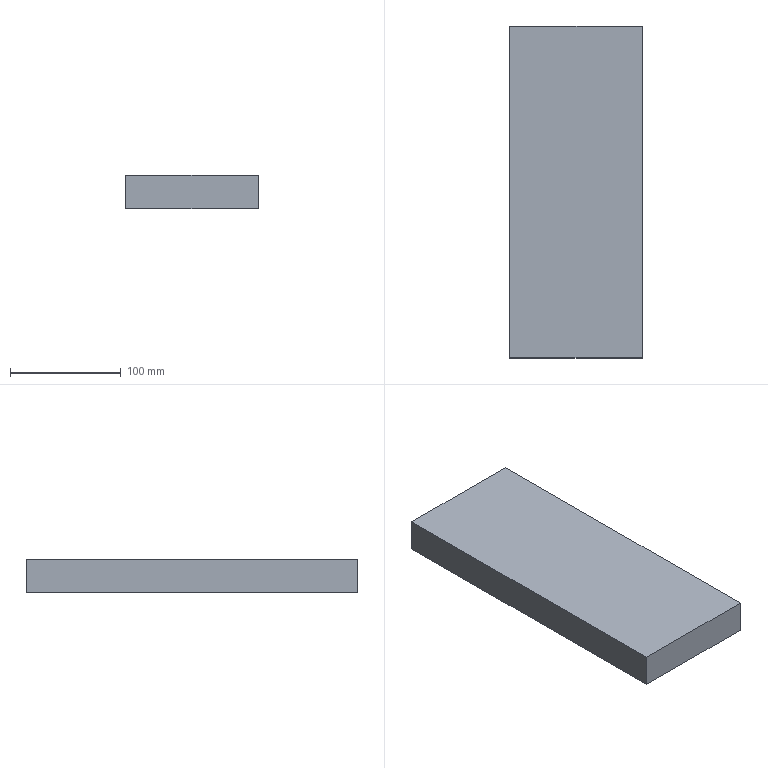Part | SolidWorks | features Extrusion 1 | 1 solid | 6 faces | box 120 x 300 x 30 mm | volume 1080000 mm3 | plane 6
STEP:
#1=CARTESIAN_POINT('',(0.,300.,0.));
#2=VERTEX_POINT('',#1);
#3=CARTESIAN_POINT('',(0.,0.,0.));
#4=VERTEX_POINT('',#3);
#5=CARTESIAN_POINT('',(0.,0.,0.));
#6=DIRECTION('',(0.,-1.,0.));
#7=VECTOR('',#6,1000.);
#8=LINE('',#5,#7);
#9=EDGE_CURVE('',#2,#4,#8,.T.);
#10=ORIENTED_EDGE('',*,*,#9,.T.);
#11=CARTESIAN_POINT('',(0.,0.,30.));
#12=VERTEX_POINT('',#11);
#13=CARTESIAN_POINT('',(0.,0.,30.));
#14=DIRECTION('',(0.,0.,-1.));
#15=VECTOR('',#14,1000.);
#16=LINE('',#13,#15);
#17=EDGE_CURVE('',#12,#4,#16,.T.);
#18=ORIENTED_EDGE('',*,*,#17,.F.);
#19=CARTESIAN_POINT('',(0.,300.,30.));
#20=VERTEX_POINT('',#19);
#21=CARTESIAN_POINT('',(0.,0.,30.));
#22=DIRECTION('',(0.,-1.,0.));
#23=VECTOR('',#22,1000.);
#24=LINE('',#21,#23);
#25=EDGE_CURVE('',#20,#12,#24,.T.);
#26=ORIENTED_EDGE('',*,*,#25,.F.);
#27=CARTESIAN_POINT('',(0.,300.,30.));
#28=DIRECTION('',(0.,0.,-1.));
#29=VECTOR('',#28,1000.);
#30=LINE('',#27,#29);
#31=EDGE_CURVE('',#20,#2,#30,.T.);
#32=ORIENTED_EDGE('',*,*,#31,.T.);
#33=EDGE_LOOP('',(#10,#18,#26,#32));
#34=FACE_OUTER_BOUND('',#33,.T.);
#35=CARTESIAN_POINT('',(0.,0.,30.));
#36=DIRECTION('',(1.,0.,0.));
#37=DIRECTION('',(0.,1.,0.));
#38=AXIS2_PLACEMENT_3D('',#35,#36,#37);
#39=PLANE('',#38);
#40=ADVANCED_FACE('',(#34),#39,.F.);
#41=CARTESIAN_POINT('',(120.,0.,0.));
#42=VERTEX_POINT('',#41);
#43=CARTESIAN_POINT('',(0.,0.,0.));
#44=DIRECTION('',(1.,0.,0.));
#45=VECTOR('',#44,1000.);
#46=LINE('',#43,#45);
#47=EDGE_CURVE('',#4,#42,#46,.T.);
#48=ORIENTED_EDGE('',*,*,#47,.T.);
#49=CARTESIAN_POINT('',(120.,0.,30.));
#50=VERTEX_POINT('',#49);
#51=CARTESIAN_POINT('',(120.,0.,30.));
#52=DIRECTION('',(0.,0.,-1.));
#53=VECTOR('',#52,1000.);
#54=LINE('',#51,#53);
#55=EDGE_CURVE('',#50,#42,#54,.T.);
#56=ORIENTED_EDGE('',*,*,#55,.F.);
#57=CARTESIAN_POINT('',(0.,0.,30.));
#58=DIRECTION('',(1.,0.,0.));
#59=VECTOR('',#58,1000.);
#60=LINE('',#57,#59);
#61=EDGE_CURVE('',#12,#50,#60,.T.);
#62=ORIENTED_EDGE('',*,*,#61,.F.);
#63=ORIENTED_EDGE('',*,*,#17,.T.);
#64=EDGE_LOOP('',(#48,#56,#62,#63));
#65=FACE_OUTER_BOUND('',#64,.T.);
#66=CARTESIAN_POINT('',(0.,0.,30.));
#67=DIRECTION('',(0.,1.,0.));
#68=DIRECTION('',(0.,0.,1.));
#69=AXIS2_PLACEMENT_3D('',#66,#67,#68);
#70=PLANE('',#69);
#71=ADVANCED_FACE('',(#65),#70,.F.);
#72=CARTESIAN_POINT('',(120.,300.,0.));
#73=VERTEX_POINT('',#72);
#74=CARTESIAN_POINT('',(120.,0.,0.));
#75=DIRECTION('',(0.,1.,0.));
#76=VECTOR('',#75,1000.);
#77=LINE('',#74,#76);
#78=EDGE_CURVE('',#42,#73,#77,.T.);
#79=ORIENTED_EDGE('',*,*,#78,.T.);
#80=CARTESIAN_POINT('',(120.,300.,30.));
#81=VERTEX_POINT('',#80);
#82=CARTESIAN_POINT('',(120.,300.,30.));
#83=DIRECTION('',(0.,0.,-1.));
#84=VECTOR('',#83,1000.);
#85=LINE('',#82,#84);
#86=EDGE_CURVE('',#81,#73,#85,.T.);
#87=ORIENTED_EDGE('',*,*,#86,.F.);
#88=CARTESIAN_POINT('',(120.,0.,30.));
#89=DIRECTION('',(0.,1.,0.));
#90=VECTOR('',#89,1000.);
#91=LINE('',#88,#90);
#92=EDGE_CURVE('',#50,#81,#91,.T.);
#93=ORIENTED_EDGE('',*,*,#92,.F.);
#94=ORIENTED_EDGE('',*,*,#55,.T.);
#95=EDGE_LOOP('',(#79,#87,#93,#94));
#96=FACE_OUTER_BOUND('',#95,.T.);
#97=CARTESIAN_POINT('',(120.,0.,30.));
#98=DIRECTION('',(-1.,0.,0.));
#99=DIRECTION('',(0.,-1.,0.));
#100=AXIS2_PLACEMENT_3D('',#97,#98,#99);
#101=PLANE('',#100);
#102=ADVANCED_FACE('',(#96),#101,.F.);
#103=CARTESIAN_POINT('',(0.,300.,0.));
#104=DIRECTION('',(-1.,0.,0.));
#105=VECTOR('',#104,1000.);
#106=LINE('',#103,#105);
#107=EDGE_CURVE('',#73,#2,#106,.T.);
#108=ORIENTED_EDGE('',*,*,#107,.T.);
#109=ORIENTED_EDGE('',*,*,#31,.F.);
#110=CARTESIAN_POINT('',(0.,300.,30.));
#111=DIRECTION('',(-1.,0.,0.));
#112=VECTOR('',#111,1000.);
#113=LINE('',#110,#112);
#114=EDGE_CURVE('',#81,#20,#113,.T.);
#115=ORIENTED_EDGE('',*,*,#114,.F.);
#116=ORIENTED_EDGE('',*,*,#86,.T.);
#117=EDGE_LOOP('',(#108,#109,#115,#116));
#118=FACE_OUTER_BOUND('',#117,.T.);
#119=CARTESIAN_POINT('',(0.,300.,30.));
#120=DIRECTION('',(0.,-1.,0.));
#121=DIRECTION('',(0.,0.,-1.));
#122=AXIS2_PLACEMENT_3D('',#119,#120,#121);
#123=PLANE('',#122);
#124=ADVANCED_FACE('',(#118),#123,.F.);
#125=ORIENTED_EDGE('',*,*,#25,.T.);
#126=ORIENTED_EDGE('',*,*,#61,.T.);
#127=ORIENTED_EDGE('',*,*,#92,.T.);
#128=ORIENTED_EDGE('',*,*,#114,.T.);
#129=EDGE_LOOP('',(#125,#126,#127,#128));
#130=FACE_OUTER_BOUND('',#129,.T.);
#131=CARTESIAN_POINT('',(0.,0.,30.));
#132=DIRECTION('',(0.,0.,-1.));
#133=DIRECTION('',(-1.,0.,0.));
#134=AXIS2_PLACEMENT_3D('',#131,#132,#133);
#135=PLANE('',#134);
#136=ADVANCED_FACE('',(#130),#135,.F.);
#137=ORIENTED_EDGE('',*,*,#9,.F.);
#138=ORIENTED_EDGE('',*,*,#107,.F.);
#139=ORIENTED_EDGE('',*,*,#78,.F.);
#140=ORIENTED_EDGE('',*,*,#47,.F.);
#141=EDGE_LOOP('',(#137,#138,#139,#140));
#142=FACE_OUTER_BOUND('',#141,.T.);
#143=CARTESIAN_POINT('',(0.,0.,0.));
#144=DIRECTION('',(0.,0.,-1.));
#145=DIRECTION('',(-1.,0.,0.));
#146=AXIS2_PLACEMENT_3D('',#143,#144,#145);
#147=PLANE('',#146);
#148=ADVANCED_FACE('',(#142),#147,.T.);
#149=CLOSED_SHELL('',(#40,#71,#102,#124,#136,#148));
#150=MANIFOLD_SOLID_BREP('',#149);
#151=CARTESIAN_POINT('',(0.,0.,0.));
#152=DIRECTION('',(0.,0.,1.));
#153=DIRECTION('',(1.,0.,0.));
#154=AXIS2_PLACEMENT_3D('',#151,#152,#153);
#155=(LENGTH_UNIT()NAMED_UNIT(*)SI_UNIT(.MILLI.,.METRE.));
#156=UNCERTAINTY_MEASURE_WITH_UNIT(LENGTH_MEASURE(0.00001),#155,'','');
#157=(NAMED_UNIT(*)PLANE_ANGLE_UNIT()SI_UNIT($,.RADIAN.));
#158=(NAMED_UNIT(*)SI_UNIT($,.STERADIAN.)SOLID_ANGLE_UNIT());
#159=(GEOMETRIC_REPRESENTATION_CONTEXT(3)GLOBAL_UNCERTAINTY_ASSIGNED_CONTEXT((#156))GLOBAL_UNIT_ASSIGNED_CONTEXT((#155,#157,#158))REPRESENTATION_CONTEXT('',''));
#160=ADVANCED_BREP_SHAPE_REPRESENTATION('',(#150,#154),#159);